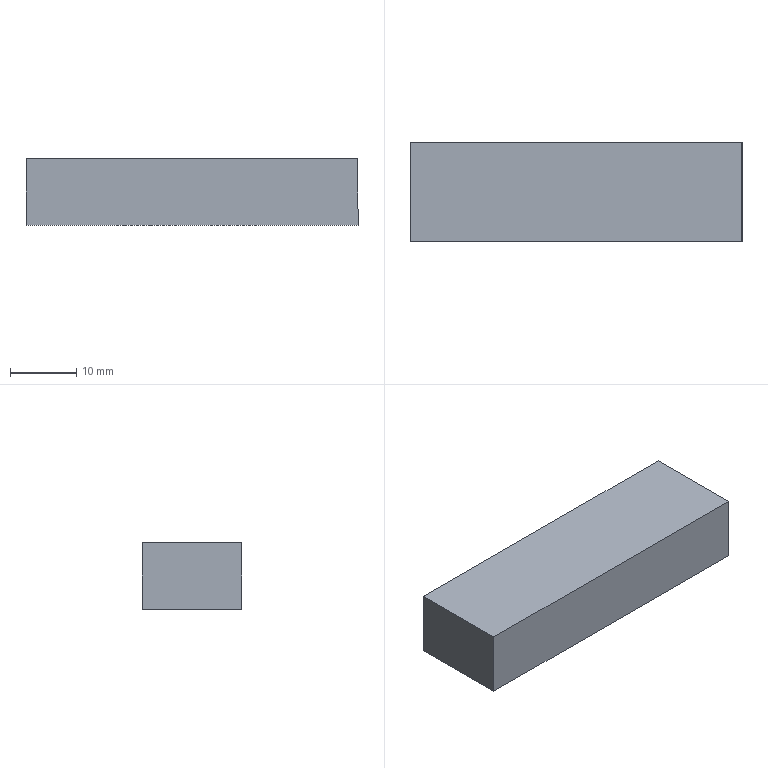NC program | NX | posted by the shop | part box 50 x 15 x 10 mm
Whole program:
%
G40 G17 G49 G80 G90
(缂栫▼浜猴細鏉庡啗浜®)
M05
M09
G91 G28 Z0.0
M01
T01 M06
S4500 M03
(ToolName=D8-25-D8-60-3T-rough D.=8.00 R.=0.00)
 (-1.50)(0.05)
G00 G90 G54 X32.5 Y0.0
T02
G43 Z20. H01 M08
Z5.638
G01 Z2.638 F1200.
X18.5
X-22.5
X-36.5
Z5.638
G00 Z20.
X32.5
Z4.775
G01 Z1.775
X18.5
X-22.5
X-36.5
Z4.775
G00 Z20.
X32.5
Z3.913
G01 Z.913
X18.5
X-22.5
X-36.5
Z3.913
G00 Z20.
X32.5
Z3.05
G01 Z.05
X18.5
X-22.5
X-36.5
Z3.05
G00 Z20.
G00 X-23.5 Y-6.964 S4500 M03
Z0.0
G01 Z-1. F2000.
Y-2.5
Y2.5
Y6.964
Z0.0
G00 Z20.
X-24.5 Y-6.972
Z-1.
G01 Z-2.
Y-2.5
Y2.5
Y6.972
Z-1.
G00 Z20.
X-25.5 Y-6.963
Z-2.
G01 Z-3.
Y-2.5
Y2.5
Y6.965
Z-2.
G00 Z20.
M05
M09
G91 G28 Z0.0
M01
T02 M06
S4500 M03
(ToolName=D8-25-D8-60-3T-finish D.=8.00 R.=0.00)
 (-1.50)(0.00)
G00 G90 G54 X32.5 Y0.0
T10
G43 Z20. H02 M08
Z3.
G01 Z0.0 F800.
X18.5
X-22.5
X-36.5
Z3.
G00 Z20.
M05
M09
G91 G28 Z0.0
M01
T10 M06
S3000 M03
(ToolName=倒角D10-90度 D.=10.00 R.=0.00)
 (-4.00)(0.00)
G00 G90 G54 X-23. Y-8.9
T01
G43 Z20. H10 M08
Z-2.5
G01 Z-4.5 F300.
Y-2.4
Y2.4
Y8.9
Z-2.5
G00 Z20.
G00 X-22. Y4. S4500 M03
Z1.5
G01 Z-1.5 F1000.
X-18.5
X18.5
G02 X20. Y2.5 I0.0 J-1.5
G01 Y-2.5
G02 X18.5 Y-4. I-1.5 J0.0
G01 X-18.5
X-22.
Z1.5
G00 Z20.
M05
M09
G91 G28 Z0.0
G28 Y0.0
M30
(The Sum of Machine Time:0.59 Minutes)
%